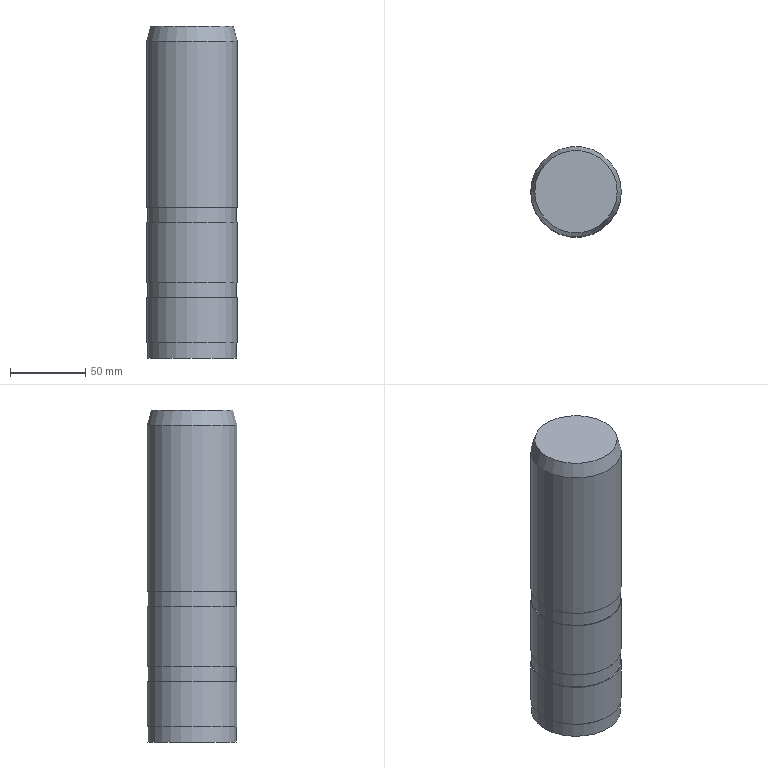Part | NX | features solid 2 | 1 solid | 14 faces | box 60 x 60 x 220 mm | volume 616781 mm3 | plane 7 | cylinder 6 | cone 1 | commonest cylinder face diameters 59 x3 60 x3
STEP:
#1=CARTESIAN_POINT('',(1149.5,310.,-285.));
#2=VERTEX_POINT('',#1);
#3=CARTESIAN_POINT('',(1120.,310.,-285.));
#4=DIRECTION('',(0.,0.,1.));
#5=DIRECTION('',(1.,0.,0.));
#6=AXIS2_PLACEMENT_3D('',#3,#4,#5);
#7=CIRCLE('',#6,29.5);
#8=EDGE_CURVE('',#2,#2,#7,.T.);
#9=ORIENTED_EDGE('',*,*,#8,.F.);
#10=EDGE_LOOP('',(#9));
#11=FACE_BOUND('',#10,.T.);
#12=CARTESIAN_POINT('',(1149.5,310.,-295.));
#13=VERTEX_POINT('',#12);
#14=CARTESIAN_POINT('',(1120.,310.,-295.));
#15=DIRECTION('',(0.,0.,1.));
#16=DIRECTION('',(1.,0.,0.));
#17=AXIS2_PLACEMENT_3D('',#14,#15,#16);
#18=CIRCLE('',#17,29.5);
#19=EDGE_CURVE('',#13,#13,#18,.T.);
#20=ORIENTED_EDGE('',*,*,#19,.T.);
#21=EDGE_LOOP('',(#20));
#22=FACE_BOUND('',#21,.T.);
#23=CARTESIAN_POINT('',(1120.,310.,-285.));
#24=DIRECTION('',(0.,0.,-1.));
#25=DIRECTION('',(-1.,0.,0.));
#26=AXIS2_PLACEMENT_3D('',#23,#24,#25);
#27=CYLINDRICAL_SURFACE('',#26,29.5);
#28=ADVANCED_FACE('',(#11,#22),#27,.T.);
#29=CARTESIAN_POINT('',(1150.,310.,-285.));
#30=VERTEX_POINT('',#29);
#31=CARTESIAN_POINT('',(1120.,310.,-285.));
#32=DIRECTION('',(0.,0.,1.));
#33=DIRECTION('',(1.,0.,0.));
#34=AXIS2_PLACEMENT_3D('',#31,#32,#33);
#35=CIRCLE('',#34,30.);
#36=EDGE_CURVE('',#30,#30,#35,.T.);
#37=ORIENTED_EDGE('',*,*,#36,.F.);
#38=EDGE_LOOP('',(#37));
#39=FACE_BOUND('',#38,.T.);
#40=ORIENTED_EDGE('',*,*,#8,.T.);
#41=EDGE_LOOP('',(#40));
#42=FACE_BOUND('',#41,.T.);
#43=CARTESIAN_POINT('',(1120.,310.,-285.));
#44=DIRECTION('',(0.,0.,1.));
#45=DIRECTION('',(1.,0.,0.));
#46=AXIS2_PLACEMENT_3D('',#43,#44,#45);
#47=PLANE('',#46);
#48=ADVANCED_FACE('',(#39,#42),#47,.F.);
#49=CARTESIAN_POINT('',(1150.,310.,-175.));
#50=VERTEX_POINT('',#49);
#51=CARTESIAN_POINT('',(1120.,310.,-175.));
#52=DIRECTION('',(0.,0.,1.));
#53=DIRECTION('',(1.,0.,0.));
#54=AXIS2_PLACEMENT_3D('',#51,#52,#53);
#55=CIRCLE('',#54,30.);
#56=EDGE_CURVE('',#50,#50,#55,.T.);
#57=ORIENTED_EDGE('',*,*,#56,.F.);
#58=EDGE_LOOP('',(#57));
#59=FACE_BOUND('',#58,.T.);
#60=ORIENTED_EDGE('',*,*,#36,.T.);
#61=EDGE_LOOP('',(#60));
#62=FACE_BOUND('',#61,.T.);
#63=CARTESIAN_POINT('',(1120.,310.,-195.));
#64=DIRECTION('',(0.,0.,-1.));
#65=DIRECTION('',(-1.,0.,0.));
#66=AXIS2_PLACEMENT_3D('',#63,#64,#65);
#67=CYLINDRICAL_SURFACE('',#66,30.);
#68=ADVANCED_FACE('',(#59,#62),#67,.T.);
#69=CARTESIAN_POINT('',(1147.321,310.,-165.));
#70=VERTEX_POINT('',#69);
#71=CARTESIAN_POINT('',(1120.,310.,-165.));
#72=DIRECTION('',(0.,0.,1.));
#73=DIRECTION('',(1.,0.,0.));
#74=AXIS2_PLACEMENT_3D('',#71,#72,#73);
#75=CIRCLE('',#74,27.321);
#76=EDGE_CURVE('',#70,#70,#75,.T.);
#77=ORIENTED_EDGE('',*,*,#76,.F.);
#78=EDGE_LOOP('',(#77));
#79=FACE_BOUND('',#78,.T.);
#80=ORIENTED_EDGE('',*,*,#56,.T.);
#81=EDGE_LOOP('',(#80));
#82=FACE_BOUND('',#81,.T.);
#83=CARTESIAN_POINT('',(1120.,310.,-175.));
#84=DIRECTION('',(0.,0.,-1.));
#85=DIRECTION('',(1.,0.,0.));
#86=AXIS2_PLACEMENT_3D('',#83,#84,#85);
#87=CONICAL_SURFACE('',#86,30.,0.2618);
#88=ADVANCED_FACE('',(#79,#82),#87,.T.);
#89=ORIENTED_EDGE('',*,*,#76,.T.);
#90=EDGE_LOOP('',(#89));
#91=FACE_BOUND('',#90,.T.);
#92=CARTESIAN_POINT('',(1120.,310.,-165.));
#93=DIRECTION('',(0.,0.,1.));
#94=DIRECTION('',(1.,0.,0.));
#95=AXIS2_PLACEMENT_3D('',#92,#93,#94);
#96=PLANE('',#95);
#97=ADVANCED_FACE('',(#91),#96,.T.);
#98=CARTESIAN_POINT('',(1150.,310.,-295.));
#99=VERTEX_POINT('',#98);
#100=CARTESIAN_POINT('',(1120.,310.,-295.));
#101=DIRECTION('',(0.,0.,1.));
#102=DIRECTION('',(1.,0.,0.));
#103=AXIS2_PLACEMENT_3D('',#100,#101,#102);
#104=CIRCLE('',#103,30.);
#105=EDGE_CURVE('',#99,#99,#104,.T.);
#106=ORIENTED_EDGE('',*,*,#105,.T.);
#107=EDGE_LOOP('',(#106));
#108=FACE_BOUND('',#107,.T.);
#109=ORIENTED_EDGE('',*,*,#19,.F.);
#110=EDGE_LOOP('',(#109));
#111=FACE_BOUND('',#110,.T.);
#112=CARTESIAN_POINT('',(1120.,310.,-295.));
#113=DIRECTION('',(0.,0.,1.));
#114=DIRECTION('',(1.,0.,0.));
#115=AXIS2_PLACEMENT_3D('',#112,#113,#114);
#116=PLANE('',#115);
#117=ADVANCED_FACE('',(#108,#111),#116,.T.);
#118=CARTESIAN_POINT('',(1150.,310.,-335.));
#119=VERTEX_POINT('',#118);
#120=CARTESIAN_POINT('',(1120.,310.,-335.));
#121=DIRECTION('',(0.,0.,1.));
#122=DIRECTION('',(1.,0.,0.));
#123=AXIS2_PLACEMENT_3D('',#120,#121,#122);
#124=CIRCLE('',#123,30.);
#125=EDGE_CURVE('',#119,#119,#124,.T.);
#126=ORIENTED_EDGE('',*,*,#125,.T.);
#127=EDGE_LOOP('',(#126));
#128=FACE_BOUND('',#127,.T.);
#129=ORIENTED_EDGE('',*,*,#105,.F.);
#130=EDGE_LOOP('',(#129));
#131=FACE_BOUND('',#130,.T.);
#132=CARTESIAN_POINT('',(1120.,310.,-335.));
#133=DIRECTION('',(0.,0.,1.));
#134=DIRECTION('',(1.,0.,0.));
#135=AXIS2_PLACEMENT_3D('',#132,#133,#134);
#136=CYLINDRICAL_SURFACE('',#135,30.);
#137=ADVANCED_FACE('',(#128,#131),#136,.T.);
#138=CARTESIAN_POINT('',(1149.5,310.,-335.));
#139=VERTEX_POINT('',#138);
#140=CARTESIAN_POINT('',(1120.,310.,-335.));
#141=DIRECTION('',(0.,0.,1.));
#142=DIRECTION('',(1.,0.,0.));
#143=AXIS2_PLACEMENT_3D('',#140,#141,#142);
#144=CIRCLE('',#143,29.5);
#145=EDGE_CURVE('',#139,#139,#144,.T.);
#146=ORIENTED_EDGE('',*,*,#145,.T.);
#147=EDGE_LOOP('',(#146));
#148=FACE_BOUND('',#147,.T.);
#149=ORIENTED_EDGE('',*,*,#125,.F.);
#150=EDGE_LOOP('',(#149));
#151=FACE_BOUND('',#150,.T.);
#152=CARTESIAN_POINT('',(1120.,310.,-335.));
#153=DIRECTION('',(0.,0.,1.));
#154=DIRECTION('',(1.,0.,0.));
#155=AXIS2_PLACEMENT_3D('',#152,#153,#154);
#156=PLANE('',#155);
#157=ADVANCED_FACE('',(#148,#151),#156,.F.);
#158=CARTESIAN_POINT('',(1149.5,310.,-345.));
#159=VERTEX_POINT('',#158);
#160=CARTESIAN_POINT('',(1120.,310.,-345.));
#161=DIRECTION('',(0.,0.,1.));
#162=DIRECTION('',(1.,0.,0.));
#163=AXIS2_PLACEMENT_3D('',#160,#161,#162);
#164=CIRCLE('',#163,29.5);
#165=EDGE_CURVE('',#159,#159,#164,.F.);
#166=ORIENTED_EDGE('',*,*,#165,.F.);
#167=EDGE_LOOP('',(#166));
#168=FACE_BOUND('',#167,.T.);
#169=ORIENTED_EDGE('',*,*,#145,.F.);
#170=EDGE_LOOP('',(#169));
#171=FACE_BOUND('',#170,.T.);
#172=CARTESIAN_POINT('',(1120.,310.,-345.));
#173=DIRECTION('',(0.,0.,1.));
#174=DIRECTION('',(1.,0.,0.));
#175=AXIS2_PLACEMENT_3D('',#172,#173,#174);
#176=CYLINDRICAL_SURFACE('',#175,29.5);
#177=ADVANCED_FACE('',(#168,#171),#176,.T.);
#178=CARTESIAN_POINT('',(1150.,310.,-375.));
#179=VERTEX_POINT('',#178);
#180=CARTESIAN_POINT('',(1120.,310.,-375.));
#181=DIRECTION('',(0.,0.,1.));
#182=DIRECTION('',(1.,0.,0.));
#183=AXIS2_PLACEMENT_3D('',#180,#181,#182);
#184=CIRCLE('',#183,30.);
#185=EDGE_CURVE('',#179,#179,#184,.T.);
#186=ORIENTED_EDGE('',*,*,#185,.T.);
#187=EDGE_LOOP('',(#186));
#188=FACE_BOUND('',#187,.T.);
#189=CARTESIAN_POINT('',(1150.,310.,-345.));
#190=VERTEX_POINT('',#189);
#191=CARTESIAN_POINT('',(1120.,310.,-345.));
#192=DIRECTION('',(0.,0.,1.));
#193=DIRECTION('',(1.,0.,0.));
#194=AXIS2_PLACEMENT_3D('',#191,#192,#193);
#195=CIRCLE('',#194,30.);
#196=EDGE_CURVE('',#190,#190,#195,.T.);
#197=ORIENTED_EDGE('',*,*,#196,.F.);
#198=EDGE_LOOP('',(#197));
#199=FACE_BOUND('',#198,.T.);
#200=CARTESIAN_POINT('',(1120.,310.,-375.));
#201=DIRECTION('',(0.,0.,1.));
#202=DIRECTION('',(1.,0.,0.));
#203=AXIS2_PLACEMENT_3D('',#200,#201,#202);
#204=CYLINDRICAL_SURFACE('',#203,30.);
#205=ADVANCED_FACE('',(#188,#199),#204,.T.);
#206=CARTESIAN_POINT('',(1149.5,310.,-375.));
#207=VERTEX_POINT('',#206);
#208=CARTESIAN_POINT('',(1120.,310.,-375.));
#209=DIRECTION('',(0.,0.,1.));
#210=DIRECTION('',(1.,0.,0.));
#211=AXIS2_PLACEMENT_3D('',#208,#209,#210);
#212=CIRCLE('',#211,29.5);
#213=EDGE_CURVE('',#207,#207,#212,.T.);
#214=ORIENTED_EDGE('',*,*,#213,.T.);
#215=EDGE_LOOP('',(#214));
#216=FACE_BOUND('',#215,.T.);
#217=ORIENTED_EDGE('',*,*,#185,.F.);
#218=EDGE_LOOP('',(#217));
#219=FACE_BOUND('',#218,.T.);
#220=CARTESIAN_POINT('',(1120.,310.,-375.));
#221=DIRECTION('',(0.,0.,1.));
#222=DIRECTION('',(1.,0.,0.));
#223=AXIS2_PLACEMENT_3D('',#220,#221,#222);
#224=PLANE('',#223);
#225=ADVANCED_FACE('',(#216,#219),#224,.F.);
#226=ORIENTED_EDGE('',*,*,#165,.T.);
#227=EDGE_LOOP('',(#226));
#228=FACE_BOUND('',#227,.T.);
#229=ORIENTED_EDGE('',*,*,#196,.T.);
#230=EDGE_LOOP('',(#229));
#231=FACE_BOUND('',#230,.T.);
#232=CARTESIAN_POINT('',(1120.,310.,-345.));
#233=DIRECTION('',(0.,0.,1.));
#234=DIRECTION('',(1.,0.,0.));
#235=AXIS2_PLACEMENT_3D('',#232,#233,#234);
#236=PLANE('',#235);
#237=ADVANCED_FACE('',(#228,#231),#236,.T.);
#238=CARTESIAN_POINT('',(1149.5,310.,-385.));
#239=VERTEX_POINT('',#238);
#240=CARTESIAN_POINT('',(1120.,310.,-385.));
#241=DIRECTION('',(0.,0.,1.));
#242=DIRECTION('',(1.,0.,0.));
#243=AXIS2_PLACEMENT_3D('',#240,#241,#242);
#244=CIRCLE('',#243,29.5);
#245=EDGE_CURVE('',#239,#239,#244,.T.);
#246=ORIENTED_EDGE('',*,*,#245,.T.);
#247=EDGE_LOOP('',(#246));
#248=FACE_BOUND('',#247,.T.);
#249=ORIENTED_EDGE('',*,*,#213,.F.);
#250=EDGE_LOOP('',(#249));
#251=FACE_BOUND('',#250,.T.);
#252=CARTESIAN_POINT('',(1120.,310.,-385.));
#253=DIRECTION('',(0.,0.,1.));
#254=DIRECTION('',(1.,0.,0.));
#255=AXIS2_PLACEMENT_3D('',#252,#253,#254);
#256=CYLINDRICAL_SURFACE('',#255,29.5);
#257=ADVANCED_FACE('',(#248,#251),#256,.T.);
#258=ORIENTED_EDGE('',*,*,#245,.F.);
#259=EDGE_LOOP('',(#258));
#260=FACE_BOUND('',#259,.T.);
#261=CARTESIAN_POINT('',(1120.,310.,-385.));
#262=DIRECTION('',(0.,0.,1.));
#263=DIRECTION('',(1.,0.,0.));
#264=AXIS2_PLACEMENT_3D('',#261,#262,#263);
#265=PLANE('',#264);
#266=ADVANCED_FACE('',(#260),#265,.F.);
#267=CLOSED_SHELL('',(#28,#48,#68,#88,#97,#117,#137,#157,#177,#205,#225,#237,#257,#266));
#268=MANIFOLD_SOLID_BREP('',#267);
#269=(LENGTH_UNIT()NAMED_UNIT(*)SI_UNIT(.MILLI.,.METRE.));
#270=UNCERTAINTY_MEASURE_WITH_UNIT(LENGTH_MEASURE(0.00001),#269,'','');
#271=(NAMED_UNIT(*)PLANE_ANGLE_UNIT()SI_UNIT($,.RADIAN.));
#272=(NAMED_UNIT(*)SI_UNIT($,.STERADIAN.)SOLID_ANGLE_UNIT());
#273=(GEOMETRIC_REPRESENTATION_CONTEXT(3)GLOBAL_UNCERTAINTY_ASSIGNED_CONTEXT((#270))GLOBAL_UNIT_ASSIGNED_CONTEXT((#269,#271,#272))REPRESENTATION_CONTEXT('',''));
#274=ADVANCED_BREP_SHAPE_REPRESENTATION('',(#268),#273);